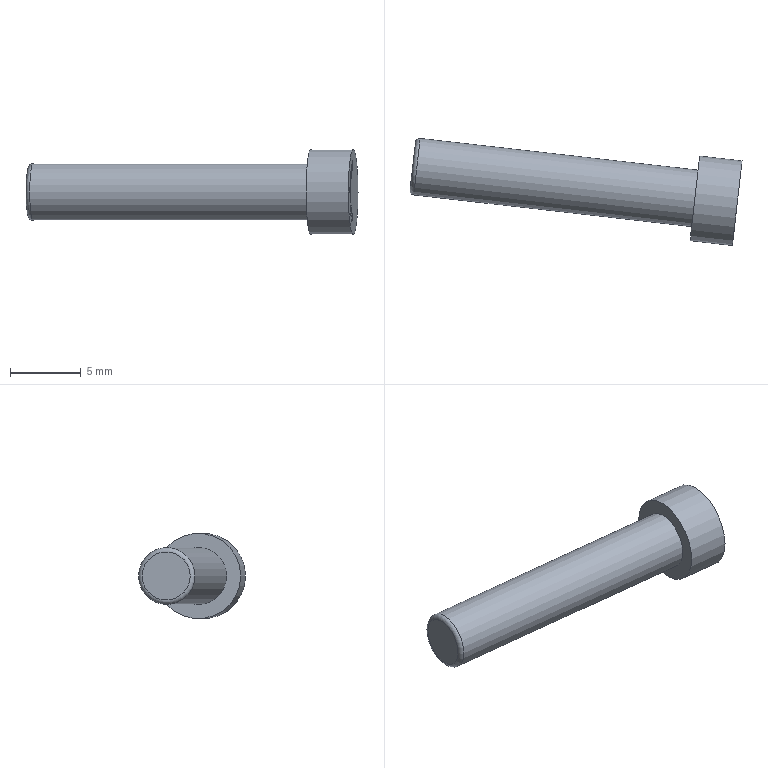Part | NX | features XQ 2 | 1 solid | 87 faces | box 23.386 x 7.54 x 6 mm | volume 335.672 mm3 | plane 63 | spline 21 | cylinder 2 | torus 1 | commonest cylinder face diameters 4 x1 6 x1